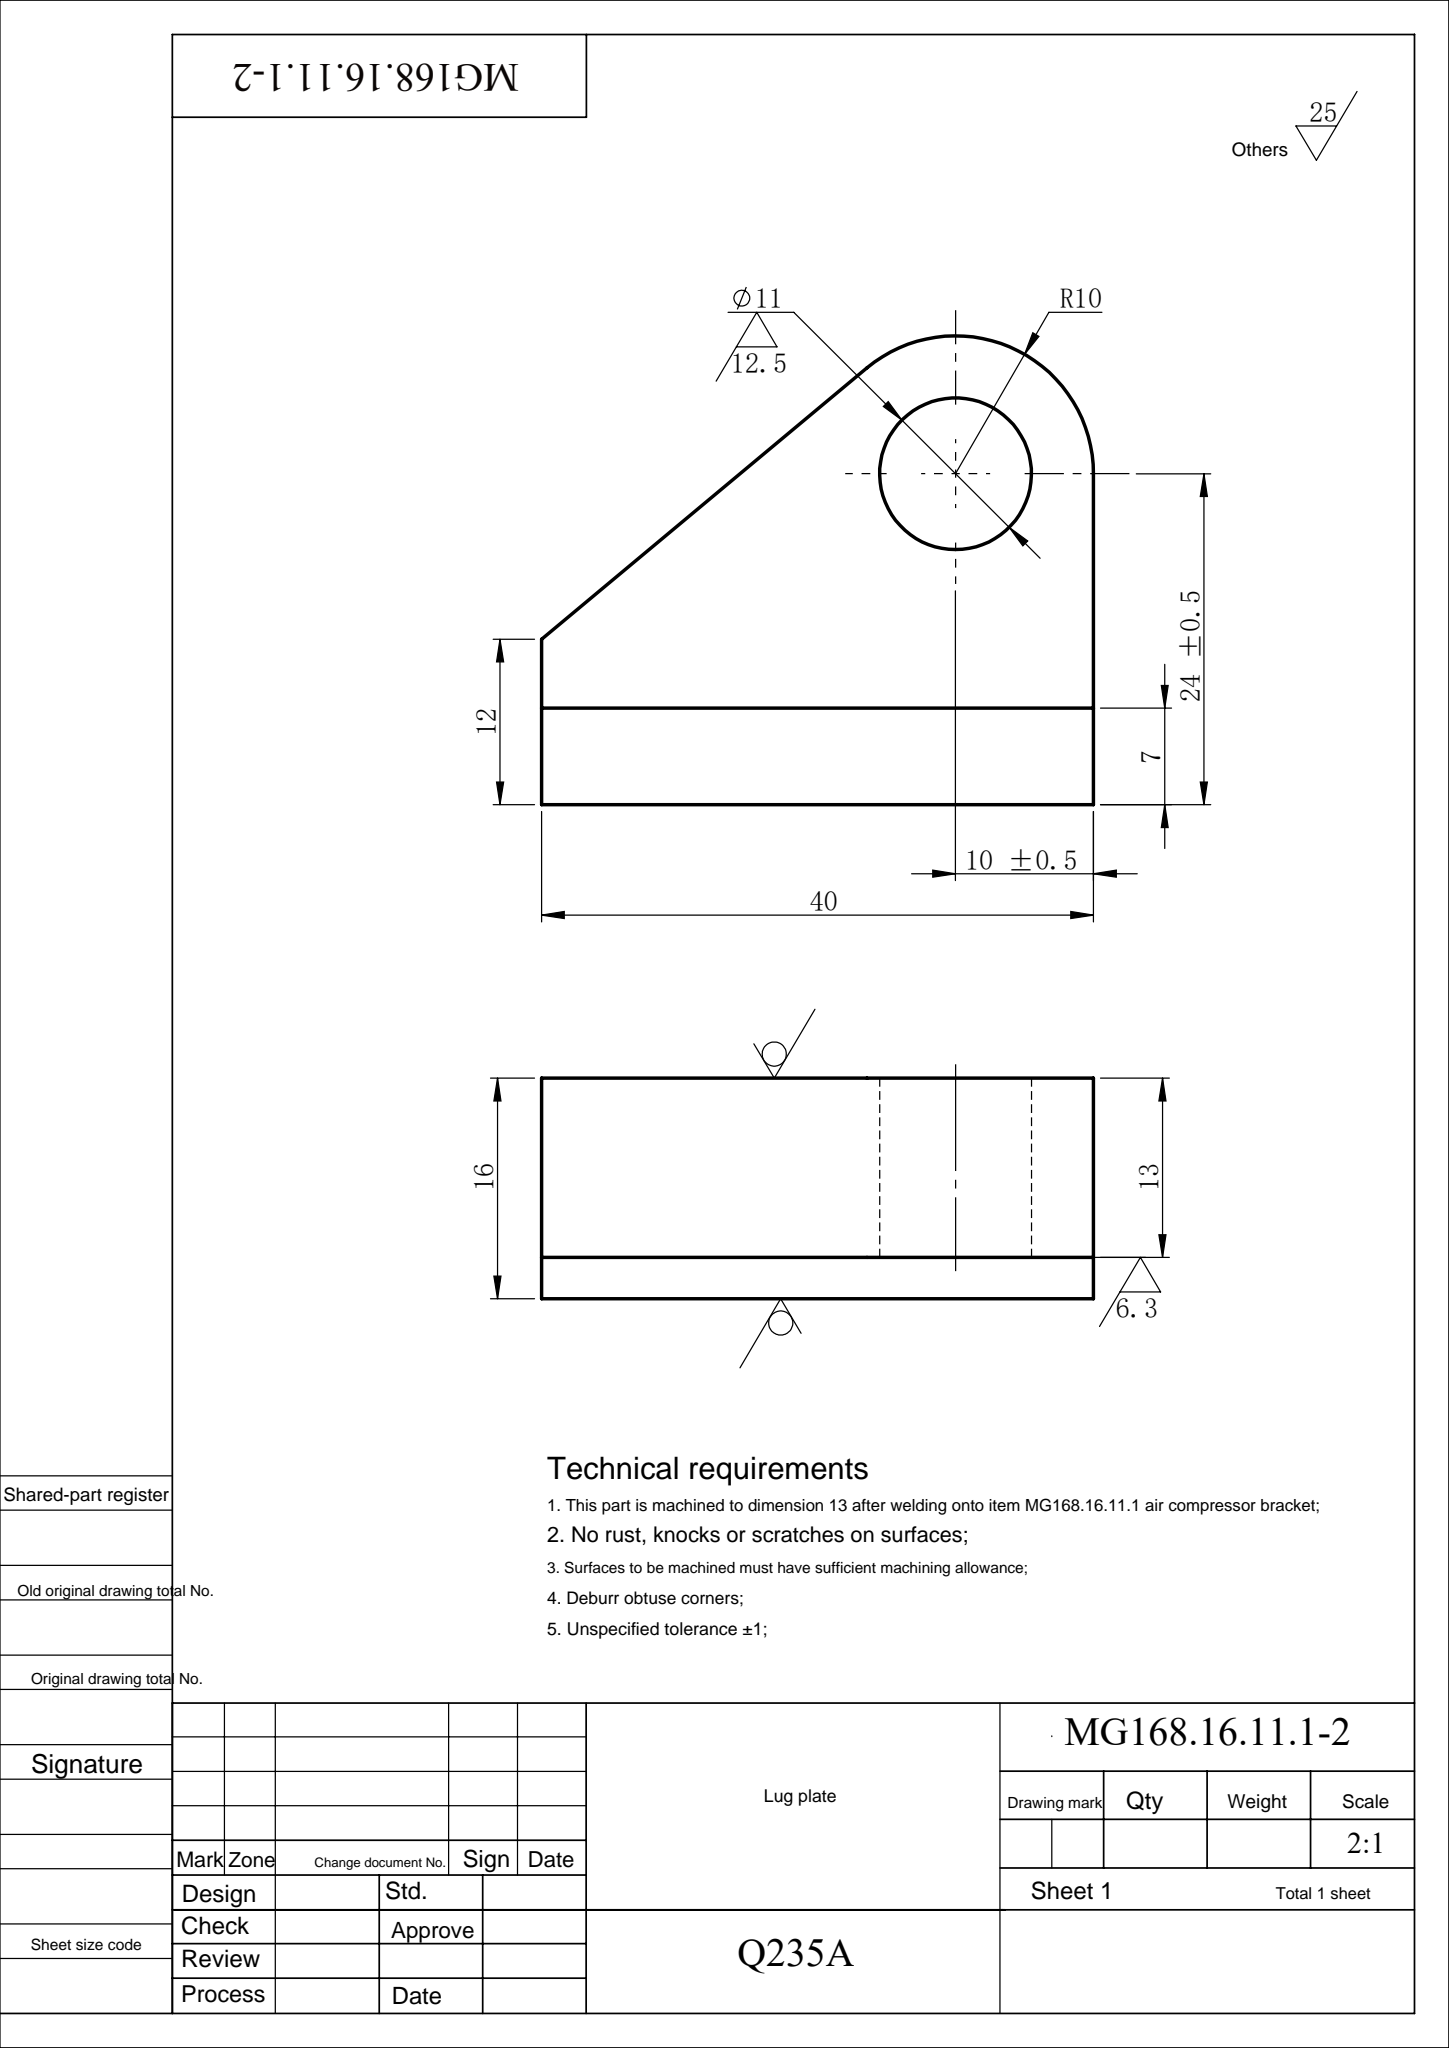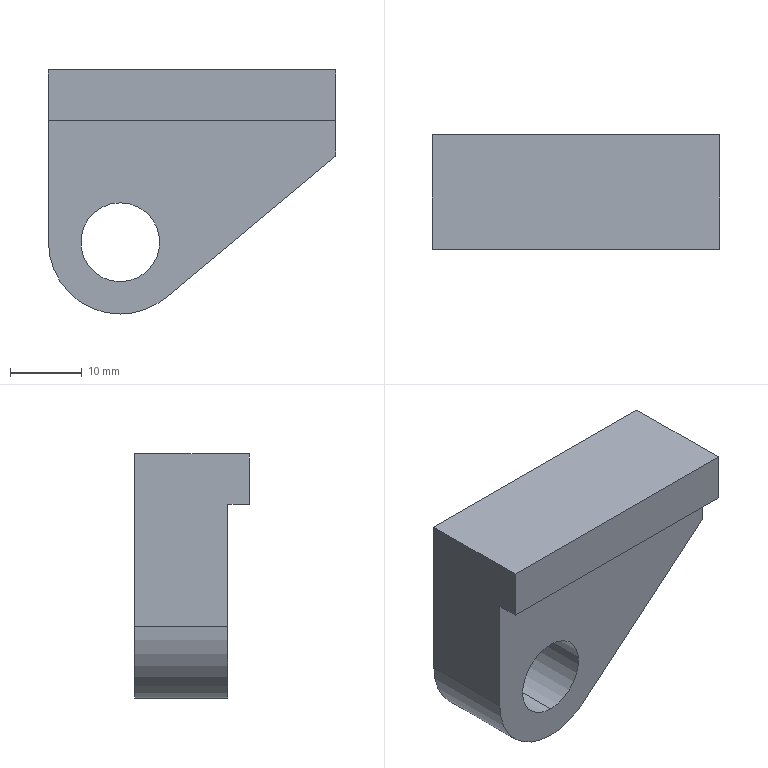Part | SolidWorks | features Extrusion 1, ICE 1 | 1 solid | 12 faces | box 40 x 16 x 34 mm | volume 13215 mm3 | plane 8 | cylinder 4 | commonest cylinder face diameters 11 x2 20 x2
STEP:
#1=CARTESIAN_POINT('',(10.,6.5,-29.5));
#2=VERTEX_POINT('',#1);
#3=CARTESIAN_POINT('',(10.,6.5,-18.5));
#4=VERTEX_POINT('',#3);
#5=CARTESIAN_POINT('',(10.,6.5,-24.));
#6=DIRECTION('',(0.,1.,0.));
#7=DIRECTION('',(0.,0.,1.));
#8=AXIS2_PLACEMENT_3D('',#5,#6,#7);
#9=CIRCLE('',#8,5.5);
#10=EDGE_CURVE('',#2,#4,#9,.T.);
#11=ORIENTED_EDGE('',*,*,#10,.T.);
#12=CARTESIAN_POINT('',(10.,-6.5,-18.5));
#13=VERTEX_POINT('',#12);
#14=CARTESIAN_POINT('',(10.,6.5,-18.5));
#15=DIRECTION('',(0.,-1.,0.));
#16=VECTOR('',#15,1000.);
#17=LINE('',#14,#16);
#18=EDGE_CURVE('',#4,#13,#17,.T.);
#19=ORIENTED_EDGE('',*,*,#18,.T.);
#20=CARTESIAN_POINT('',(10.,-6.5,-29.5));
#21=VERTEX_POINT('',#20);
#22=CARTESIAN_POINT('',(10.,-6.5,-24.));
#23=DIRECTION('',(0.,1.,0.));
#24=DIRECTION('',(0.,0.,1.));
#25=AXIS2_PLACEMENT_3D('',#22,#23,#24);
#26=CIRCLE('',#25,5.5);
#27=EDGE_CURVE('',#21,#13,#26,.T.);
#28=ORIENTED_EDGE('',*,*,#27,.F.);
#29=CARTESIAN_POINT('',(10.,6.5,-29.5));
#30=DIRECTION('',(0.,-1.,0.));
#31=VECTOR('',#30,1000.);
#32=LINE('',#29,#31);
#33=EDGE_CURVE('',#2,#21,#32,.T.);
#34=ORIENTED_EDGE('',*,*,#33,.F.);
#35=EDGE_LOOP('',(#11,#19,#28,#34));
#36=FACE_OUTER_BOUND('',#35,.T.);
#37=CARTESIAN_POINT('',(10.,6.5,-24.));
#38=DIRECTION('',(0.,-1.,0.));
#39=DIRECTION('',(0.,0.,-1.));
#40=AXIS2_PLACEMENT_3D('',#37,#38,#39);
#41=CYLINDRICAL_SURFACE('',#40,5.5);
#42=ADVANCED_FACE('',(#36),#41,.F.);
#43=CARTESIAN_POINT('',(10.,6.5,-34.));
#44=VERTEX_POINT('',#43);
#45=CARTESIAN_POINT('',(0.,6.5,-24.));
#46=VERTEX_POINT('',#45);
#47=CARTESIAN_POINT('',(10.,6.5,-24.));
#48=DIRECTION('',(0.,1.,0.));
#49=DIRECTION('',(0.,0.,-1.));
#50=AXIS2_PLACEMENT_3D('',#47,#48,#49);
#51=CIRCLE('',#50,10.);
#52=EDGE_CURVE('',#44,#46,#51,.T.);
#53=ORIENTED_EDGE('',*,*,#52,.F.);
#54=CARTESIAN_POINT('',(10.,-6.5,-34.));
#55=VERTEX_POINT('',#54);
#56=CARTESIAN_POINT('',(10.,6.5,-34.));
#57=DIRECTION('',(0.,-1.,0.));
#58=VECTOR('',#57,1000.);
#59=LINE('',#56,#58);
#60=EDGE_CURVE('',#44,#55,#59,.T.);
#61=ORIENTED_EDGE('',*,*,#60,.T.);
#62=CARTESIAN_POINT('',(0.,-6.5,-24.));
#63=VERTEX_POINT('',#62);
#64=CARTESIAN_POINT('',(10.,-6.5,-24.));
#65=DIRECTION('',(0.,1.,0.));
#66=DIRECTION('',(0.,0.,-1.));
#67=AXIS2_PLACEMENT_3D('',#64,#65,#66);
#68=CIRCLE('',#67,10.);
#69=EDGE_CURVE('',#55,#63,#68,.T.);
#70=ORIENTED_EDGE('',*,*,#69,.T.);
#71=CARTESIAN_POINT('',(0.,6.5,-24.));
#72=DIRECTION('',(0.,-1.,0.));
#73=VECTOR('',#72,1000.);
#74=LINE('',#71,#73);
#75=EDGE_CURVE('',#46,#63,#74,.T.);
#76=ORIENTED_EDGE('',*,*,#75,.F.);
#77=EDGE_LOOP('',(#53,#61,#70,#76));
#78=FACE_OUTER_BOUND('',#77,.T.);
#79=CARTESIAN_POINT('',(10.,6.5,-24.));
#80=DIRECTION('',(0.,-1.,0.));
#81=DIRECTION('',(0.,0.,-1.));
#82=AXIS2_PLACEMENT_3D('',#79,#80,#81);
#83=CYLINDRICAL_SURFACE('',#82,10.);
#84=ADVANCED_FACE('',(#78),#83,.T.);
#85=ORIENTED_EDGE('',*,*,#27,.T.);
#86=CARTESIAN_POINT('',(10.,-6.5,-24.));
#87=DIRECTION('',(0.,1.,0.));
#88=DIRECTION('',(0.,0.,1.));
#89=AXIS2_PLACEMENT_3D('',#86,#87,#88);
#90=CIRCLE('',#89,5.5);
#91=EDGE_CURVE('',#13,#21,#90,.T.);
#92=ORIENTED_EDGE('',*,*,#91,.T.);
#93=EDGE_LOOP('',(#85,#92));
#94=FACE_BOUND('',#93,.T.);
#95=CARTESIAN_POINT('',(40.,-6.5,-7.));
#96=VERTEX_POINT('',#95);
#97=CARTESIAN_POINT('',(40.,-6.5,-12.));
#98=VERTEX_POINT('',#97);
#99=CARTESIAN_POINT('',(40.,-6.5,0.));
#100=DIRECTION('',(0.,0.,-1.));
#101=VECTOR('',#100,1000.);
#102=LINE('',#99,#101);
#103=EDGE_CURVE('',#96,#98,#102,.T.);
#104=ORIENTED_EDGE('',*,*,#103,.F.);
#105=CARTESIAN_POINT('',(0.,-6.5,-7.));
#106=VERTEX_POINT('',#105);
#107=CARTESIAN_POINT('',(0.,-6.5,-7.));
#108=DIRECTION('',(-1.,0.,0.));
#109=VECTOR('',#108,1000.);
#110=LINE('',#107,#109);
#111=EDGE_CURVE('',#96,#106,#110,.T.);
#112=ORIENTED_EDGE('',*,*,#111,.T.);
#113=CARTESIAN_POINT('',(0.,-6.5,0.));
#114=DIRECTION('',(0.,0.,1.));
#115=VECTOR('',#114,1000.);
#116=LINE('',#113,#115);
#117=EDGE_CURVE('',#63,#106,#116,.T.);
#118=ORIENTED_EDGE('',*,*,#117,.F.);
#119=ORIENTED_EDGE('',*,*,#69,.F.);
#120=CARTESIAN_POINT('',(16.405,-6.5,-31.679));
#121=VERTEX_POINT('',#120);
#122=CARTESIAN_POINT('',(10.,-6.5,-24.));
#123=DIRECTION('',(0.,1.,0.));
#124=DIRECTION('',(0.,0.,-1.));
#125=AXIS2_PLACEMENT_3D('',#122,#123,#124);
#126=CIRCLE('',#125,10.);
#127=EDGE_CURVE('',#121,#55,#126,.T.);
#128=ORIENTED_EDGE('',*,*,#127,.F.);
#129=CARTESIAN_POINT('',(40.,-6.5,-12.));
#130=DIRECTION('',(-0.7679,0.,-0.6405));
#131=VECTOR('',#130,1000.);
#132=LINE('',#129,#131);
#133=EDGE_CURVE('',#98,#121,#132,.T.);
#134=ORIENTED_EDGE('',*,*,#133,.F.);
#135=EDGE_LOOP('',(#104,#112,#118,#119,#128,#134));
#136=FACE_OUTER_BOUND('',#135,.T.);
#137=CARTESIAN_POINT('',(10.,-6.5,-24.));
#138=DIRECTION('',(0.,-1.,0.));
#139=DIRECTION('',(0.,0.,-1.));
#140=AXIS2_PLACEMENT_3D('',#137,#138,#139);
#141=PLANE('',#140);
#142=ADVANCED_FACE('',(#94,#136),#141,.T.);
#143=CARTESIAN_POINT('',(0.,6.5,0.));
#144=VERTEX_POINT('',#143);
#145=CARTESIAN_POINT('',(0.,6.5,0.));
#146=DIRECTION('',(0.,0.,1.));
#147=VECTOR('',#146,1000.);
#148=LINE('',#145,#147);
#149=EDGE_CURVE('',#46,#144,#148,.T.);
#150=ORIENTED_EDGE('',*,*,#149,.T.);
#151=CARTESIAN_POINT('',(40.,6.5,0.));
#152=VERTEX_POINT('',#151);
#153=CARTESIAN_POINT('',(0.,6.5,0.));
#154=DIRECTION('',(1.,0.,0.));
#155=VECTOR('',#154,1000.);
#156=LINE('',#153,#155);
#157=EDGE_CURVE('',#144,#152,#156,.T.);
#158=ORIENTED_EDGE('',*,*,#157,.T.);
#159=CARTESIAN_POINT('',(40.,6.5,-12.));
#160=VERTEX_POINT('',#159);
#161=CARTESIAN_POINT('',(40.,6.5,0.));
#162=DIRECTION('',(0.,0.,-1.));
#163=VECTOR('',#162,1000.);
#164=LINE('',#161,#163);
#165=EDGE_CURVE('',#152,#160,#164,.T.);
#166=ORIENTED_EDGE('',*,*,#165,.T.);
#167=CARTESIAN_POINT('',(16.405,6.5,-31.679));
#168=VERTEX_POINT('',#167);
#169=CARTESIAN_POINT('',(40.,6.5,-12.));
#170=DIRECTION('',(-0.7679,0.,-0.6405));
#171=VECTOR('',#170,1000.);
#172=LINE('',#169,#171);
#173=EDGE_CURVE('',#160,#168,#172,.T.);
#174=ORIENTED_EDGE('',*,*,#173,.T.);
#175=CARTESIAN_POINT('',(10.,6.5,-24.));
#176=DIRECTION('',(0.,1.,0.));
#177=DIRECTION('',(0.,0.,-1.));
#178=AXIS2_PLACEMENT_3D('',#175,#176,#177);
#179=CIRCLE('',#178,10.);
#180=EDGE_CURVE('',#168,#44,#179,.T.);
#181=ORIENTED_EDGE('',*,*,#180,.T.);
#182=ORIENTED_EDGE('',*,*,#52,.T.);
#183=EDGE_LOOP('',(#150,#158,#166,#174,#181,#182));
#184=FACE_OUTER_BOUND('',#183,.T.);
#185=ORIENTED_EDGE('',*,*,#10,.F.);
#186=CARTESIAN_POINT('',(10.,6.5,-24.));
#187=DIRECTION('',(0.,1.,0.));
#188=DIRECTION('',(0.,0.,1.));
#189=AXIS2_PLACEMENT_3D('',#186,#187,#188);
#190=CIRCLE('',#189,5.5);
#191=EDGE_CURVE('',#4,#2,#190,.T.);
#192=ORIENTED_EDGE('',*,*,#191,.F.);
#193=EDGE_LOOP('',(#185,#192));
#194=FACE_BOUND('',#193,.T.);
#195=CARTESIAN_POINT('',(10.,6.5,-24.));
#196=DIRECTION('',(0.,-1.,0.));
#197=DIRECTION('',(0.,0.,-1.));
#198=AXIS2_PLACEMENT_3D('',#195,#196,#197);
#199=PLANE('',#198);
#200=ADVANCED_FACE('',(#184,#194),#199,.F.);
#201=ORIENTED_EDGE('',*,*,#117,.T.);
#202=CARTESIAN_POINT('',(0.,-9.5,-7.));
#203=VERTEX_POINT('',#202);
#204=CARTESIAN_POINT('',(0.,-9.5,-7.));
#205=DIRECTION('',(0.,1.,0.));
#206=VECTOR('',#205,1000.);
#207=LINE('',#204,#206);
#208=EDGE_CURVE('',#203,#106,#207,.T.);
#209=ORIENTED_EDGE('',*,*,#208,.F.);
#210=CARTESIAN_POINT('',(0.,-9.5,0.));
#211=VERTEX_POINT('',#210);
#212=CARTESIAN_POINT('',(0.,-9.5,0.));
#213=DIRECTION('',(0.,0.,1.));
#214=VECTOR('',#213,1000.);
#215=LINE('',#212,#214);
#216=EDGE_CURVE('',#203,#211,#215,.T.);
#217=ORIENTED_EDGE('',*,*,#216,.T.);
#218=CARTESIAN_POINT('',(0.,6.5,0.));
#219=DIRECTION('',(0.,-1.,0.));
#220=VECTOR('',#219,1000.);
#221=LINE('',#218,#220);
#222=EDGE_CURVE('',#144,#211,#221,.T.);
#223=ORIENTED_EDGE('',*,*,#222,.F.);
#224=ORIENTED_EDGE('',*,*,#149,.F.);
#225=ORIENTED_EDGE('',*,*,#75,.T.);
#226=EDGE_LOOP('',(#201,#209,#217,#223,#224,#225));
#227=FACE_OUTER_BOUND('',#226,.T.);
#228=CARTESIAN_POINT('',(0.,6.5,0.));
#229=DIRECTION('',(1.,0.,0.));
#230=DIRECTION('',(0.,0.,-1.));
#231=AXIS2_PLACEMENT_3D('',#228,#229,#230);
#232=PLANE('',#231);
#233=ADVANCED_FACE('',(#227),#232,.F.);
#234=ORIENTED_EDGE('',*,*,#222,.T.);
#235=CARTESIAN_POINT('',(40.,-9.5,0.));
#236=VERTEX_POINT('',#235);
#237=CARTESIAN_POINT('',(0.,-9.5,0.));
#238=DIRECTION('',(1.,0.,0.));
#239=VECTOR('',#238,1000.);
#240=LINE('',#237,#239);
#241=EDGE_CURVE('',#211,#236,#240,.T.);
#242=ORIENTED_EDGE('',*,*,#241,.T.);
#243=CARTESIAN_POINT('',(40.,6.5,0.));
#244=DIRECTION('',(0.,-1.,0.));
#245=VECTOR('',#244,1000.);
#246=LINE('',#243,#245);
#247=EDGE_CURVE('',#152,#236,#246,.T.);
#248=ORIENTED_EDGE('',*,*,#247,.F.);
#249=ORIENTED_EDGE('',*,*,#157,.F.);
#250=EDGE_LOOP('',(#234,#242,#248,#249));
#251=FACE_OUTER_BOUND('',#250,.T.);
#252=CARTESIAN_POINT('',(0.,6.5,0.));
#253=DIRECTION('',(0.,0.,-1.));
#254=DIRECTION('',(-1.,0.,0.));
#255=AXIS2_PLACEMENT_3D('',#252,#253,#254);
#256=PLANE('',#255);
#257=ADVANCED_FACE('',(#251),#256,.F.);
#258=ORIENTED_EDGE('',*,*,#247,.T.);
#259=CARTESIAN_POINT('',(40.,-9.5,-7.));
#260=VERTEX_POINT('',#259);
#261=CARTESIAN_POINT('',(40.,-9.5,0.));
#262=DIRECTION('',(0.,0.,-1.));
#263=VECTOR('',#262,1000.);
#264=LINE('',#261,#263);
#265=EDGE_CURVE('',#236,#260,#264,.T.);
#266=ORIENTED_EDGE('',*,*,#265,.T.);
#267=CARTESIAN_POINT('',(40.,-9.5,-7.));
#268=DIRECTION('',(0.,1.,0.));
#269=VECTOR('',#268,1000.);
#270=LINE('',#267,#269);
#271=EDGE_CURVE('',#260,#96,#270,.T.);
#272=ORIENTED_EDGE('',*,*,#271,.T.);
#273=ORIENTED_EDGE('',*,*,#103,.T.);
#274=CARTESIAN_POINT('',(40.,6.5,-12.));
#275=DIRECTION('',(0.,-1.,0.));
#276=VECTOR('',#275,1000.);
#277=LINE('',#274,#276);
#278=EDGE_CURVE('',#160,#98,#277,.T.);
#279=ORIENTED_EDGE('',*,*,#278,.F.);
#280=ORIENTED_EDGE('',*,*,#165,.F.);
#281=EDGE_LOOP('',(#258,#266,#272,#273,#279,#280));
#282=FACE_OUTER_BOUND('',#281,.T.);
#283=CARTESIAN_POINT('',(40.,6.5,0.));
#284=DIRECTION('',(-1.,0.,0.));
#285=DIRECTION('',(0.,0.,1.));
#286=AXIS2_PLACEMENT_3D('',#283,#284,#285);
#287=PLANE('',#286);
#288=ADVANCED_FACE('',(#282),#287,.F.);
#289=ORIENTED_EDGE('',*,*,#133,.T.);
#290=CARTESIAN_POINT('',(16.405,6.5,-31.679));
#291=DIRECTION('',(0.,-1.,0.));
#292=VECTOR('',#291,1000.);
#293=LINE('',#290,#292);
#294=EDGE_CURVE('',#168,#121,#293,.T.);
#295=ORIENTED_EDGE('',*,*,#294,.F.);
#296=ORIENTED_EDGE('',*,*,#173,.F.);
#297=ORIENTED_EDGE('',*,*,#278,.T.);
#298=EDGE_LOOP('',(#289,#295,#296,#297));
#299=FACE_OUTER_BOUND('',#298,.T.);
#300=CARTESIAN_POINT('',(40.,6.5,-12.));
#301=DIRECTION('',(-0.6405,0.,0.7679));
#302=DIRECTION('',(0.7679,0.,0.6405));
#303=AXIS2_PLACEMENT_3D('',#300,#301,#302);
#304=PLANE('',#303);
#305=ADVANCED_FACE('',(#299),#304,.F.);
#306=ORIENTED_EDGE('',*,*,#60,.F.);
#307=ORIENTED_EDGE('',*,*,#180,.F.);
#308=ORIENTED_EDGE('',*,*,#294,.T.);
#309=ORIENTED_EDGE('',*,*,#127,.T.);
#310=EDGE_LOOP('',(#306,#307,#308,#309));
#311=FACE_OUTER_BOUND('',#310,.T.);
#312=CARTESIAN_POINT('',(10.,6.5,-24.));
#313=DIRECTION('',(0.,-1.,0.));
#314=DIRECTION('',(0.,0.,-1.));
#315=AXIS2_PLACEMENT_3D('',#312,#313,#314);
#316=CYLINDRICAL_SURFACE('',#315,10.);
#317=ADVANCED_FACE('',(#311),#316,.T.);
#318=ORIENTED_EDGE('',*,*,#18,.F.);
#319=ORIENTED_EDGE('',*,*,#191,.T.);
#320=ORIENTED_EDGE('',*,*,#33,.T.);
#321=ORIENTED_EDGE('',*,*,#91,.F.);
#322=EDGE_LOOP('',(#318,#319,#320,#321));
#323=FACE_OUTER_BOUND('',#322,.T.);
#324=CARTESIAN_POINT('',(10.,6.5,-24.));
#325=DIRECTION('',(0.,-1.,0.));
#326=DIRECTION('',(0.,0.,-1.));
#327=AXIS2_PLACEMENT_3D('',#324,#325,#326);
#328=CYLINDRICAL_SURFACE('',#327,5.5);
#329=ADVANCED_FACE('',(#323),#328,.F.);
#330=ORIENTED_EDGE('',*,*,#111,.F.);
#331=ORIENTED_EDGE('',*,*,#271,.F.);
#332=CARTESIAN_POINT('',(0.,-9.5,-7.));
#333=DIRECTION('',(-1.,0.,0.));
#334=VECTOR('',#333,1000.);
#335=LINE('',#332,#334);
#336=EDGE_CURVE('',#260,#203,#335,.T.);
#337=ORIENTED_EDGE('',*,*,#336,.T.);
#338=ORIENTED_EDGE('',*,*,#208,.T.);
#339=EDGE_LOOP('',(#330,#331,#337,#338));
#340=FACE_OUTER_BOUND('',#339,.T.);
#341=CARTESIAN_POINT('',(0.,-9.5,-7.));
#342=DIRECTION('',(0.,0.,-1.));
#343=DIRECTION('',(-1.,0.,0.));
#344=AXIS2_PLACEMENT_3D('',#341,#342,#343);
#345=PLANE('',#344);
#346=ADVANCED_FACE('',(#340),#345,.T.);
#347=ORIENTED_EDGE('',*,*,#216,.F.);
#348=ORIENTED_EDGE('',*,*,#336,.F.);
#349=ORIENTED_EDGE('',*,*,#265,.F.);
#350=ORIENTED_EDGE('',*,*,#241,.F.);
#351=EDGE_LOOP('',(#347,#348,#349,#350));
#352=FACE_OUTER_BOUND('',#351,.T.);
#353=CARTESIAN_POINT('',(0.,-9.5,0.));
#354=DIRECTION('',(0.,-1.,0.));
#355=DIRECTION('',(0.,0.,-1.));
#356=AXIS2_PLACEMENT_3D('',#353,#354,#355);
#357=PLANE('',#356);
#358=ADVANCED_FACE('',(#352),#357,.T.);
#359=CLOSED_SHELL('',(#42,#84,#142,#200,#233,#257,#288,#305,#317,#329,#346,#358));
#360=MANIFOLD_SOLID_BREP('',#359);
#361=CARTESIAN_POINT('',(0.,0.,0.));
#362=DIRECTION('',(0.,0.,1.));
#363=DIRECTION('',(1.,0.,0.));
#364=AXIS2_PLACEMENT_3D('',#361,#362,#363);
#365=(LENGTH_UNIT()NAMED_UNIT(*)SI_UNIT(.MILLI.,.METRE.));
#366=UNCERTAINTY_MEASURE_WITH_UNIT(LENGTH_MEASURE(0.00001),#365,'','');
#367=(NAMED_UNIT(*)PLANE_ANGLE_UNIT()SI_UNIT($,.RADIAN.));
#368=(NAMED_UNIT(*)SI_UNIT($,.STERADIAN.)SOLID_ANGLE_UNIT());
#369=(GEOMETRIC_REPRESENTATION_CONTEXT(3)GLOBAL_UNCERTAINTY_ASSIGNED_CONTEXT((#366))GLOBAL_UNIT_ASSIGNED_CONTEXT((#365,#367,#368))REPRESENTATION_CONTEXT('',''));
#370=ADVANCED_BREP_SHAPE_REPRESENTATION('',(#360,#364),#369);